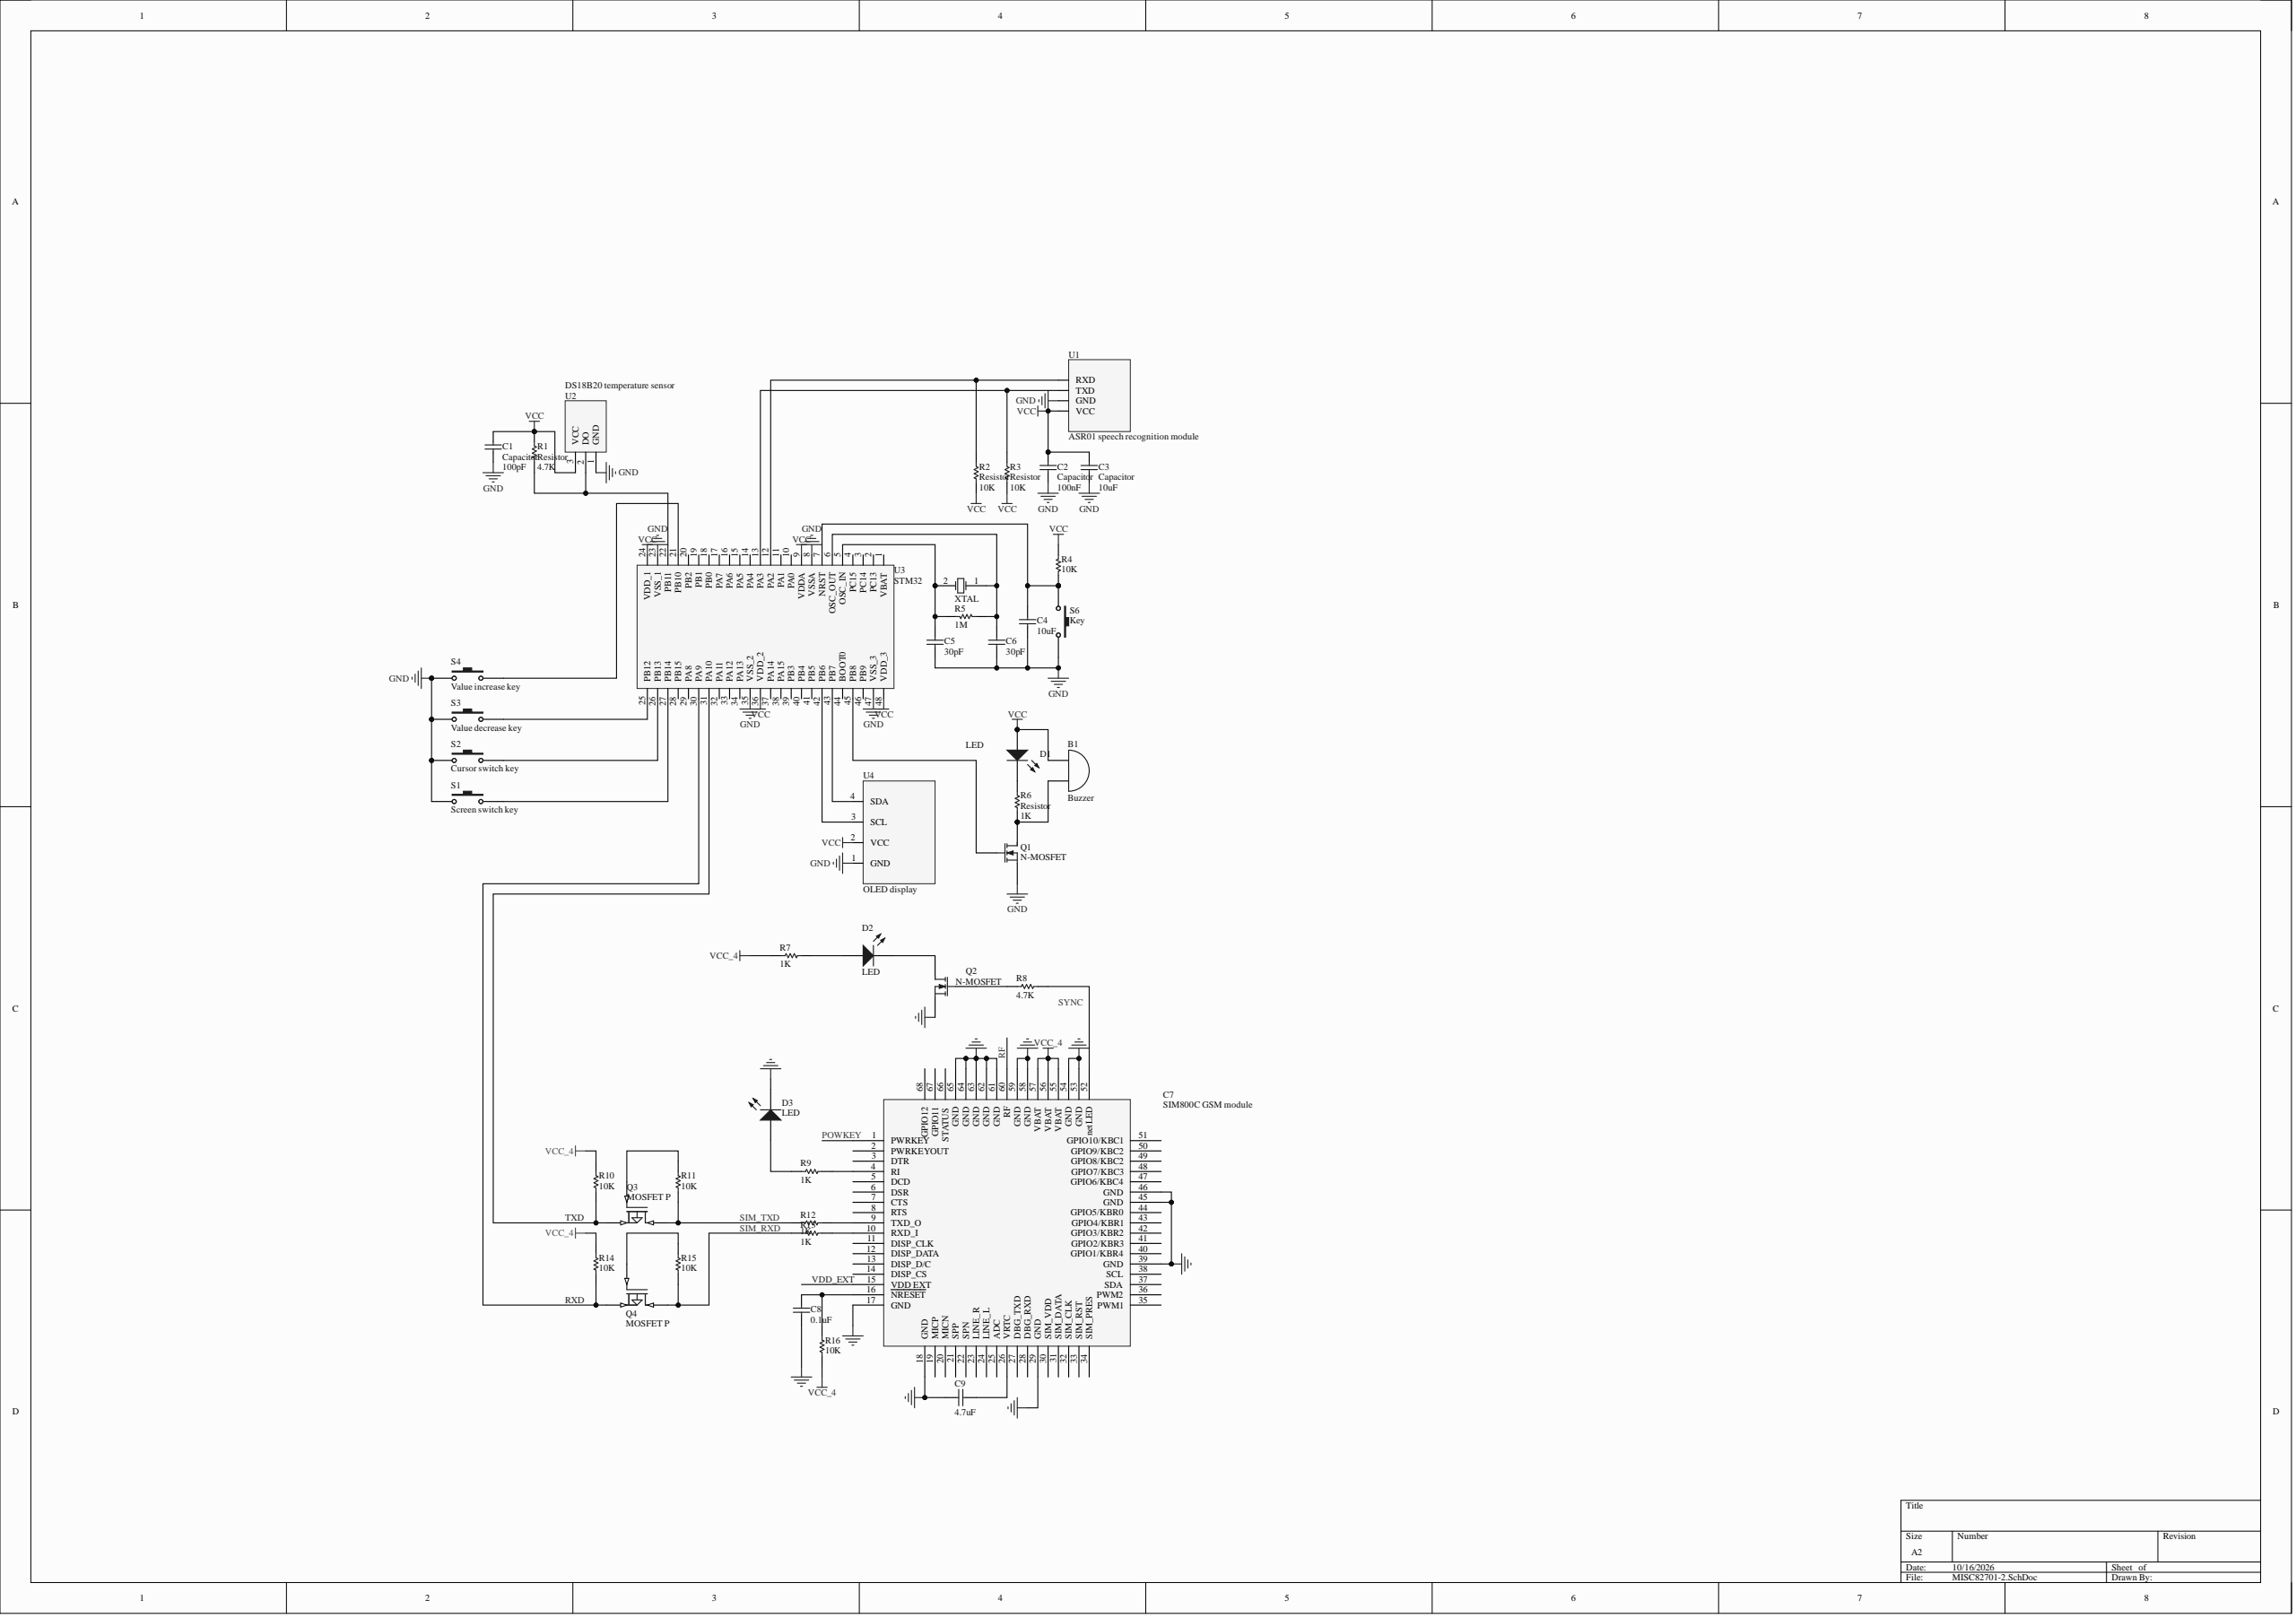Circuit board | Altium Designer | 43 parts | 34 nets
Bill of materials:
Comment,Description,Designator,Footprint,LibRef,Quantity
"Buzzer","Buzzer","B1","PIN2","蜂鸣器","1"
"Capacitor","SMD capacitor","C1, C2, C3","0603C","电容","3"
"10uF","Capacitor (Semiconductor SIM Model)","C4","0603C","Cap Semi","1"
"Cap","Capacitor","C5, C6","0603C","Cap","2"
"SIM800C GSM module","","C7","GSMM_SMD_SIM900A","SIM 900A","1"
"Capacitor","SMD capacitor","C8, C9","0805C","电容","2"
"LED","LED","D1, D2, D3","3.2X1.6X1.1","LED灯","3"
"N-MOSFET","MOSFET","Q1, Q2","SOT23","SI2302","2"
"MOSFET P","","Q3, Q4","E3","MOSFET P","2"
"Resistor","SMD resistor","R1, R2, R3, R6, R7, R8, R9, R10, R11, R12, R13, R14, R15, R16","0805R","电阻","14"
"Res Semi","Semiconductor Resistor","R4, R5","0805R","Res Semi","2"
"Screen switch key","","S1","四脚轻触开关","按键","1"
"Cursor switch key","","S2","四脚轻触开关","按键","1"
"Value decrease key","","S3","四脚轻触开关","按键","1"
"Value increase key","","S4","四脚轻触开关","按键","1"
"Key","","S6","四脚轻触开关","按键","1"
"ASR01 speech recognition module","HC-05 Bluetooth module","U1","HDR1X4","HC-05蓝牙模块_1","1"
"DS18B20 temperature sensor","Temperature sensor","U2","DS18B20","DS18B20","1"
"STM32","STM32","U3","LQFP48 7X7","STM32F103C8T6_2","1"
"OLED display","","U4","0.96OLED_4P","OLED显示器2","1"
"XTAL","Crystal Oscillator","Y1","XTAL_US","XTAL","1"
Netlist (Protel format):
[
B1
PIN2
Buzzer



]
[
C1
0603C
Capacitor



]
[
C2
0603C
Capacitor



]
[
C3
0603C
Capacitor



]
[
C4
0603C
10uF



]
[
C5
0603C
Cap



]
[
C6
0603C
Cap



]
[
C7
GSMM_SMD_SIM900A
SIM800C GSM module



]
[
C8
0805C
Capacitor



]
[
C9
0805C
Capacitor



]
[
D1
3.2X1.6X1.1
LED



]
[
D2
3.2X1.6X1.1
LED



]
[
D3
3.2X1.6X1.1
LED



]
[
Q1
SOT23
N-MOSFET



]
[
Q2
SOT23
N-MOSFET



]
[
Q3
E3
MOSFET P



]
[
Q4
E3
MOSFET P



]
[
R1
0805R
Resistor



]
[
R2
0805R
Resistor



]
[
R3
0805R
Resistor



]
[
R4
0805R
Res Semi



]
[
R5
0805R
Res Semi



]
[
R6
0805R
Resistor



]
[
R7
0805R
Resistor



]
[
R8
0805R
Resistor



]
[
R9
0805R
Resistor



]
[
R10
0805R
Resistor



]
[
R11
0805R
Resistor



]
[
R12
0805R
Resistor



]
[
R13
0805R
Resistor



]
[
R14
0805R
Resistor



]
[
R15
0805R
Resistor



]
[
R16
0805R
Resistor



]
[
S1
四脚轻触开关
Screen switch key



]
[
S2
四脚轻触开关
Cursor switch key



]
[
S3
四脚轻触开关
Value decrease key



]
[
S4
四脚轻触开关
Value increase key



]
[
S6
四脚轻触开关
Key



]
[
U1
HDR1X4
ASR01 speech recognition module



]
[
U2
DS18B20
DS18B20 temperature sensor



]
[
U3
LQFP48 7X7
STM32



]
[
U4
0.96OLED_4P
OLED display



]
[
Y1
XTAL_US
XTAL



]
(
VCC_4
C7-55
C7-56
C7-57
R7-2
R10-2
R14-2
R16-1
)
(
VCC
B1-1
C1-2
C2-1
C3-1
D1-1
R1-2
R2-2
R3-2
R4-1
U1-1
U2-3
U3-9
U3-24
U3-36
U3-48
U4-2
)
(
TXD
Q3-3
R10-1
U3-31
)
(
SIM_TXD
Q3-2
R11-1
R12-1
)
(
SIM_RXD
Q4-2
R13-1
R15-1
)
(
RXD
Q4-3
R14-1
U3-30
)
(
NetU3_43
U3-43
U4-4
)
(
NetU3_42
U3-42
U4-3
)
(
NetS4_1
S4-1
U3-21
)
(
NetS3_1
S3-1
U3-25
)
(
NetS2_1
S2-1
U3-26
)
(
NetS1_1
S1-1
U3-27
)
(
NetR3_1
R3-1
U1-3
U3-13
)
(
NetR2_1
R2-1
U1-4
U3-12
)
(
NetR1_1
R1-1
U2-2
U3-22
)
(
NetQ4_1
Q4-1
R15-2
)
(
NetQ3_1
Q3-1
R11-2
)
(
NetQ2_1
Q2-1
R8-1
)
(
NetQ1_1
Q1-1
U3-45
)
(
NetD3_1
D3-1
R9-1
)
(
NetD2_2
D2-2
Q2-3
)
(
NetD2_1
D2-1
R7-1
)
(
NetD1_2
D1-2
R6-1
)
(
NetC7_52
C7-52
R8-2
)
(
NetC7_26
C7-26
C9-1
)
(
NetC7_16
C7-16
C8-2
R16-2
)
(
NetC7_10
C7-10
R13-2
)
(
NetC7_9
C7-9
R12-2
)
(
NetC7_4
C7-4
R9-2
)
(
NetC6_1
C6-1
R5-2
U3-6
Y1-1
)
(
NetC5_1
C5-1
R5-1
U3-5
Y1-2
)
(
NetC4_1
C4-1
R4-2
S6-2
U3-7
)
(
NetB1_2
B1-2
Q1-3
R6-2
)
(
GND
C1-1
C2-2
C3-2
C4-2
C5-2
C6-2
C7-17
C7-18
C7-29
C7-39
C7-45
C7-46
C7-53
C7-54
C7-58
C7-59
C7-61
C7-62
C7-63
C7-64
C7-65
C8-1
C9-2
D3-2
Q1-2
Q2-2
S1-2
S2-2
S3-2
S4-2
S6-1
U1-2
U2-1
U3-8
U3-23
U3-35
U3-47
U4-1
)